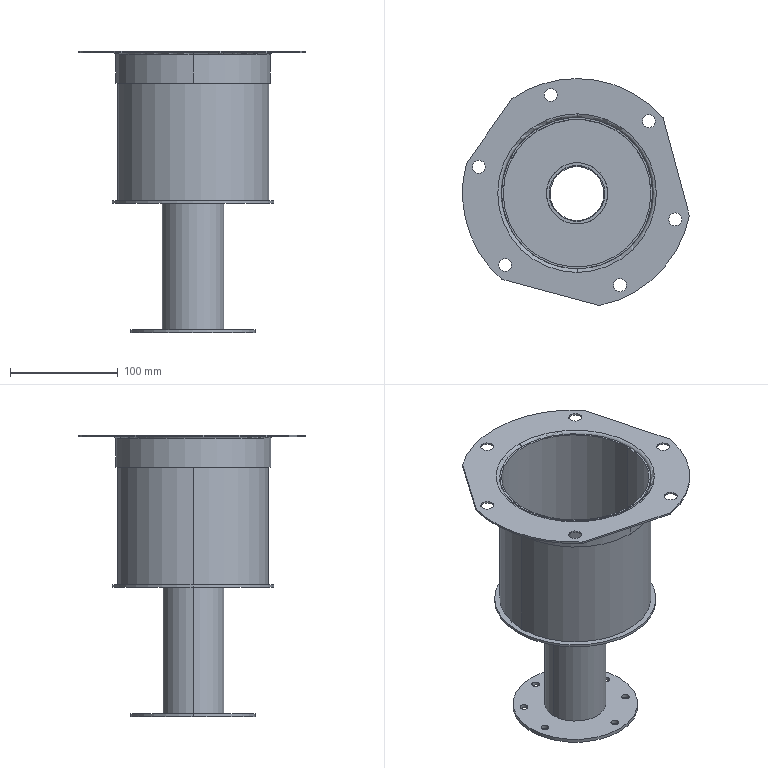Part | SolidWorks | features BaseBody 5 | 5 solids | 74 faces | box 210.893 x 210.893 x 262.1 mm | volume 260766 mm3 | cylinder 54 | plane 16 | torus 4 | commonest cylinder face diameters 7.2 x12 12 x12 4 x6 213 x4 50 x2 51.8 x2